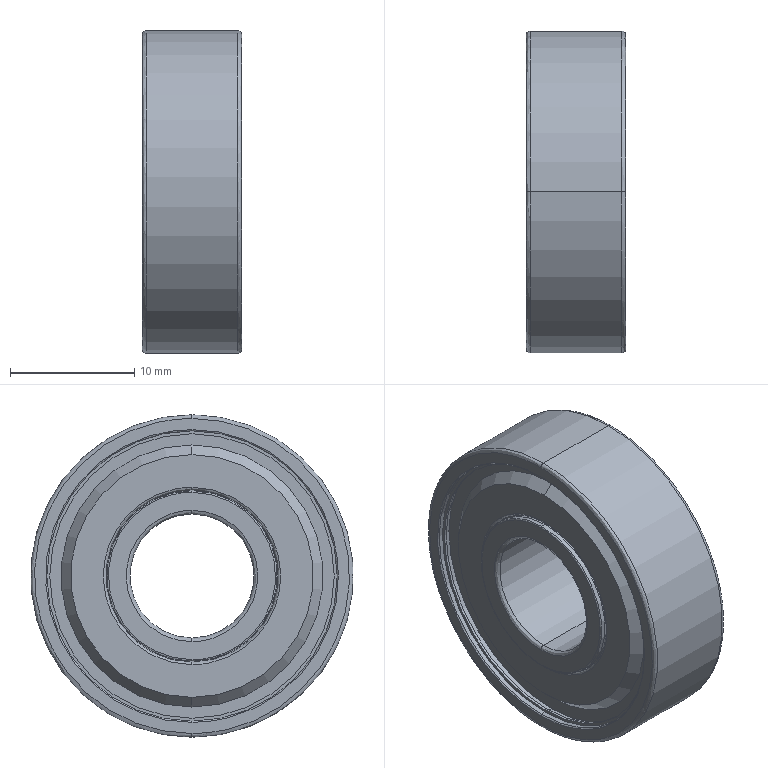Part | STEP file | Bearing B6000ZZ_MISUMI | 1 solid | 102 faces | box 8 x 26 x 26 mm | volume 2470 mm3 | spline 36 | cylinder 36 | plane 22 | cone 8 | commonest cylinder face diameters 23.4 x8 13.3 x4 13.7 x4 13.9 x4 14.3 x4 22.93 x4